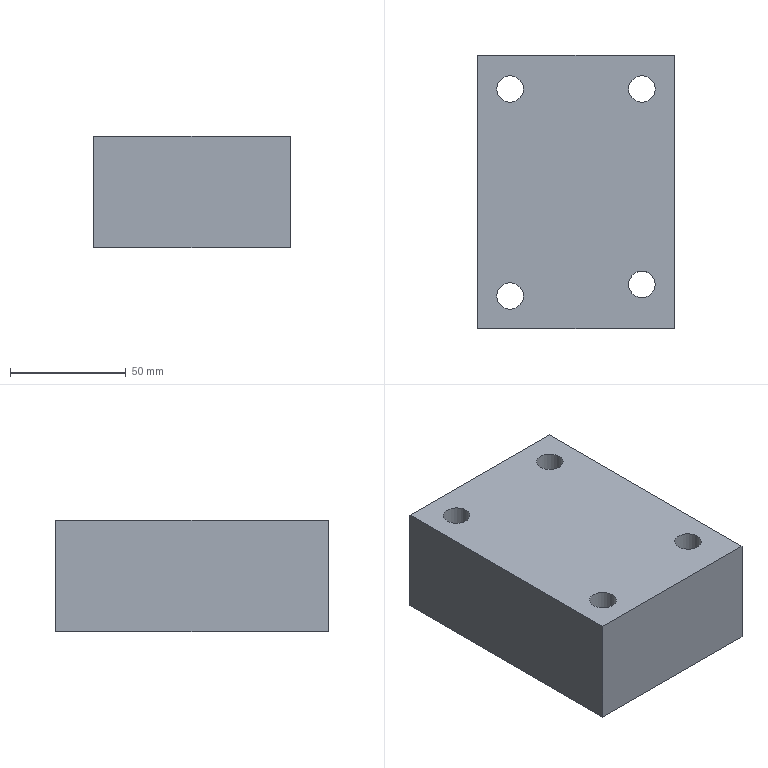Part | NX | features solid 2 | 1 solid | 35 faces | box 85 x 118 x 48 mm | volume 417820 mm3 | cylinder 16 | plane 15 | cone 4 | commonest cylinder face diameters 10 x4 11.509 x4 18.007 x4 8.5 x2 8.506 x2
STEP:
#1=CARTESIAN_POINT('',(1168.789,-205.654,50.));
#2=VERTEX_POINT('',#1);
#3=CARTESIAN_POINT('',(1159.786,-205.654,50.));
#4=DIRECTION('',(0.,0.,-1.));
#5=DIRECTION('',(1.,0.,0.));
#6=AXIS2_PLACEMENT_3D('',#3,#4,#5);
#7=CIRCLE('',#6,9.004);
#8=EDGE_CURVE('',#2,#2,#7,.T.);
#9=ORIENTED_EDGE('',*,*,#8,.F.);
#10=EDGE_LOOP('',(#9));
#11=FACE_BOUND('',#10,.T.);
#12=CARTESIAN_POINT('',(1225.789,-116.154,50.));
#13=VERTEX_POINT('',#12);
#14=CARTESIAN_POINT('',(1216.786,-116.154,50.));
#15=DIRECTION('',(0.,0.,-1.));
#16=DIRECTION('',(1.,0.,0.));
#17=AXIS2_PLACEMENT_3D('',#14,#15,#16);
#18=CIRCLE('',#17,9.004);
#19=EDGE_CURVE('',#13,#13,#18,.T.);
#20=ORIENTED_EDGE('',*,*,#19,.F.);
#21=EDGE_LOOP('',(#20));
#22=FACE_BOUND('',#21,.T.);
#23=CARTESIAN_POINT('',(1230.786,-219.654,50.));
#24=VERTEX_POINT('',#23);
#25=CARTESIAN_POINT('',(1145.786,-219.654,50.));
#26=VERTEX_POINT('',#25);
#27=CARTESIAN_POINT('',(1188.286,-219.654,50.));
#28=DIRECTION('',(-1.,0.,0.));
#29=VECTOR('',#28,1000.);
#30=LINE('',#27,#29);
#31=EDGE_CURVE('',#24,#26,#30,.T.);
#32=ORIENTED_EDGE('',*,*,#31,.T.);
#33=CARTESIAN_POINT('',(1145.786,-101.654,50.));
#34=VERTEX_POINT('',#33);
#35=CARTESIAN_POINT('',(1145.786,0.,50.));
#36=DIRECTION('',(0.,-1.,0.));
#37=VECTOR('',#36,1000.);
#38=LINE('',#35,#37);
#39=EDGE_CURVE('',#34,#26,#38,.T.);
#40=ORIENTED_EDGE('',*,*,#39,.F.);
#41=CARTESIAN_POINT('',(1230.786,-101.654,50.));
#42=VERTEX_POINT('',#41);
#43=CARTESIAN_POINT('',(1188.286,-101.654,50.));
#44=DIRECTION('',(-1.,0.,0.));
#45=VECTOR('',#44,1000.);
#46=LINE('',#43,#45);
#47=EDGE_CURVE('',#42,#34,#46,.T.);
#48=ORIENTED_EDGE('',*,*,#47,.F.);
#49=CARTESIAN_POINT('',(1230.786,0.,50.));
#50=DIRECTION('',(0.,1.,0.));
#51=VECTOR('',#50,1000.);
#52=LINE('',#49,#51);
#53=EDGE_CURVE('',#24,#42,#52,.T.);
#54=ORIENTED_EDGE('',*,*,#53,.F.);
#55=EDGE_LOOP('',(#32,#40,#48,#54));
#56=FACE_BOUND('',#55,.T.);
#57=CARTESIAN_POINT('',(1225.789,-200.654,50.));
#58=VERTEX_POINT('',#57);
#59=CARTESIAN_POINT('',(1216.786,-200.654,50.));
#60=DIRECTION('',(0.,0.,-1.));
#61=DIRECTION('',(1.,0.,0.));
#62=AXIS2_PLACEMENT_3D('',#59,#60,#61);
#63=CIRCLE('',#62,9.004);
#64=EDGE_CURVE('',#58,#58,#63,.T.);
#65=ORIENTED_EDGE('',*,*,#64,.F.);
#66=EDGE_LOOP('',(#65));
#67=FACE_BOUND('',#66,.T.);
#68=CARTESIAN_POINT('',(1168.789,-116.154,50.));
#69=VERTEX_POINT('',#68);
#70=CARTESIAN_POINT('',(1159.786,-116.154,50.));
#71=DIRECTION('',(0.,0.,-1.));
#72=DIRECTION('',(1.,0.,0.));
#73=AXIS2_PLACEMENT_3D('',#70,#71,#72);
#74=CIRCLE('',#73,9.004);
#75=EDGE_CURVE('',#69,#69,#74,.T.);
#76=ORIENTED_EDGE('',*,*,#75,.F.);
#77=EDGE_LOOP('',(#76));
#78=FACE_BOUND('',#77,.T.);
#79=CARTESIAN_POINT('',(1156.536,-159.154,50.));
#80=VERTEX_POINT('',#79);
#81=CARTESIAN_POINT('',(1160.786,-159.154,50.));
#82=DIRECTION('',(0.,0.,1.));
#83=DIRECTION('',(-1.,0.,0.));
#84=AXIS2_PLACEMENT_3D('',#81,#82,#83);
#85=CIRCLE('',#84,4.25);
#86=EDGE_CURVE('',#80,#80,#85,.T.);
#87=ORIENTED_EDGE('',*,*,#86,.T.);
#88=EDGE_LOOP('',(#87));
#89=FACE_BOUND('',#88,.T.);
#90=CARTESIAN_POINT('',(1211.536,-159.154,50.));
#91=VERTEX_POINT('',#90);
#92=CARTESIAN_POINT('',(1215.786,-159.154,50.));
#93=DIRECTION('',(0.,0.,1.));
#94=DIRECTION('',(-1.,0.,0.));
#95=AXIS2_PLACEMENT_3D('',#92,#93,#94);
#96=CIRCLE('',#95,4.25);
#97=EDGE_CURVE('',#91,#91,#96,.T.);
#98=ORIENTED_EDGE('',*,*,#97,.T.);
#99=EDGE_LOOP('',(#98));
#100=FACE_BOUND('',#99,.T.);
#101=CARTESIAN_POINT('',(1206.996,-131.014,50.));
#102=VERTEX_POINT('',#101);
#103=CARTESIAN_POINT('',(1199.996,-124.014,50.));
#104=VERTEX_POINT('',#103);
#105=CARTESIAN_POINT('',(1203.996,-127.014,50.));
#106=DIRECTION('',(0.,0.,1.));
#107=DIRECTION('',(-1.,0.,0.));
#108=AXIS2_PLACEMENT_3D('',#105,#106,#107);
#109=CIRCLE('',#108,5.);
#110=EDGE_CURVE('',#102,#104,#109,.T.);
#111=ORIENTED_EDGE('',*,*,#110,.T.);
#112=CARTESIAN_POINT('',(1176.576,-124.014,50.));
#113=VERTEX_POINT('',#112);
#114=CARTESIAN_POINT('',(1127.,-124.014,50.));
#115=DIRECTION('',(1.,0.,0.));
#116=VECTOR('',#115,1000.);
#117=LINE('',#114,#116);
#118=EDGE_CURVE('',#113,#104,#117,.T.);
#119=ORIENTED_EDGE('',*,*,#118,.F.);
#120=CARTESIAN_POINT('',(1169.576,-131.014,50.));
#121=VERTEX_POINT('',#120);
#122=CARTESIAN_POINT('',(1172.576,-127.014,50.));
#123=DIRECTION('',(0.,0.,1.));
#124=DIRECTION('',(-1.,0.,0.));
#125=AXIS2_PLACEMENT_3D('',#122,#123,#124);
#126=CIRCLE('',#125,5.);
#127=EDGE_CURVE('',#113,#121,#126,.T.);
#128=ORIENTED_EDGE('',*,*,#127,.T.);
#129=CARTESIAN_POINT('',(1169.576,-187.154,50.));
#130=VERTEX_POINT('',#129);
#131=CARTESIAN_POINT('',(1169.576,0.,50.));
#132=DIRECTION('',(0.,1.,0.));
#133=VECTOR('',#132,1000.);
#134=LINE('',#131,#133);
#135=EDGE_CURVE('',#130,#121,#134,.T.);
#136=ORIENTED_EDGE('',*,*,#135,.F.);
#137=CARTESIAN_POINT('',(1176.576,-194.154,50.));
#138=VERTEX_POINT('',#137);
#139=CARTESIAN_POINT('',(1172.576,-191.154,50.));
#140=DIRECTION('',(0.,0.,1.));
#141=DIRECTION('',(-1.,0.,0.));
#142=AXIS2_PLACEMENT_3D('',#139,#140,#141);
#143=CIRCLE('',#142,5.);
#144=EDGE_CURVE('',#130,#138,#143,.T.);
#145=ORIENTED_EDGE('',*,*,#144,.T.);
#146=CARTESIAN_POINT('',(1199.996,-194.154,50.));
#147=VERTEX_POINT('',#146);
#148=CARTESIAN_POINT('',(1127.,-194.154,50.));
#149=DIRECTION('',(-1.,0.,0.));
#150=VECTOR('',#149,1000.);
#151=LINE('',#148,#150);
#152=EDGE_CURVE('',#147,#138,#151,.T.);
#153=ORIENTED_EDGE('',*,*,#152,.F.);
#154=CARTESIAN_POINT('',(1206.996,-187.154,50.));
#155=VERTEX_POINT('',#154);
#156=CARTESIAN_POINT('',(1203.996,-191.154,50.));
#157=DIRECTION('',(0.,0.,1.));
#158=DIRECTION('',(-1.,0.,0.));
#159=AXIS2_PLACEMENT_3D('',#156,#157,#158);
#160=CIRCLE('',#159,5.);
#161=EDGE_CURVE('',#155,#147,#160,.F.);
#162=ORIENTED_EDGE('',*,*,#161,.F.);
#163=CARTESIAN_POINT('',(1206.996,0.,50.));
#164=DIRECTION('',(0.,-1.,0.));
#165=VECTOR('',#164,1000.);
#166=LINE('',#163,#165);
#167=EDGE_CURVE('',#102,#155,#166,.T.);
#168=ORIENTED_EDGE('',*,*,#167,.F.);
#169=EDGE_LOOP('',(#111,#119,#128,#136,#145,#153,#162,#168));
#170=FACE_BOUND('',#169,.T.);
#171=CARTESIAN_POINT('',(1127.,0.,50.));
#172=DIRECTION('',(0.,0.,-1.));
#173=DIRECTION('',(-1.,0.,0.));
#174=AXIS2_PLACEMENT_3D('',#171,#172,#173);
#175=PLANE('',#174);
#176=ADVANCED_FACE('',(#11,#22,#56,#67,#78,#89,#100,#170),#175,.T.);
#177=CARTESIAN_POINT('',(1230.786,-101.654,98.));
#178=VERTEX_POINT('',#177);
#179=CARTESIAN_POINT('',(1230.786,-219.654,98.));
#180=VERTEX_POINT('',#179);
#181=CARTESIAN_POINT('',(1230.786,0.,98.));
#182=DIRECTION('',(0.,-1.,0.));
#183=VECTOR('',#182,1000.);
#184=LINE('',#181,#183);
#185=EDGE_CURVE('',#178,#180,#184,.T.);
#186=ORIENTED_EDGE('',*,*,#185,.T.);
#187=CARTESIAN_POINT('',(1230.786,-219.654,-52.75));
#188=DIRECTION('',(0.,0.,-1.));
#189=VECTOR('',#188,1000.);
#190=LINE('',#187,#189);
#191=EDGE_CURVE('',#180,#24,#190,.T.);
#192=ORIENTED_EDGE('',*,*,#191,.T.);
#193=ORIENTED_EDGE('',*,*,#53,.T.);
#194=CARTESIAN_POINT('',(1230.786,-101.654,50.));
#195=DIRECTION('',(0.,0.,1.));
#196=VECTOR('',#195,1000.);
#197=LINE('',#194,#196);
#198=EDGE_CURVE('',#42,#178,#197,.T.);
#199=ORIENTED_EDGE('',*,*,#198,.T.);
#200=EDGE_LOOP('',(#186,#192,#193,#199));
#201=FACE_BOUND('',#200,.T.);
#202=CARTESIAN_POINT('',(1230.786,-216.654,50.));
#203=DIRECTION('',(1.,0.,0.));
#204=DIRECTION('',(0.,0.,-1.));
#205=AXIS2_PLACEMENT_3D('',#202,#203,#204);
#206=PLANE('',#205);
#207=ADVANCED_FACE('',(#201),#206,.T.);
#208=CARTESIAN_POINT('',(1165.54,-205.654,98.));
#209=VERTEX_POINT('',#208);
#210=CARTESIAN_POINT('',(1159.786,-205.654,98.));
#211=DIRECTION('',(0.,0.,-1.));
#212=DIRECTION('',(1.,0.,0.));
#213=AXIS2_PLACEMENT_3D('',#210,#211,#212);
#214=CIRCLE('',#213,5.755);
#215=EDGE_CURVE('',#209,#209,#214,.T.);
#216=ORIENTED_EDGE('',*,*,#215,.T.);
#217=EDGE_LOOP('',(#216));
#218=FACE_BOUND('',#217,.T.);
#219=CARTESIAN_POINT('',(1165.54,-116.154,98.));
#220=VERTEX_POINT('',#219);
#221=CARTESIAN_POINT('',(1159.786,-116.154,98.));
#222=DIRECTION('',(0.,0.,-1.));
#223=DIRECTION('',(1.,0.,0.));
#224=AXIS2_PLACEMENT_3D('',#221,#222,#223);
#225=CIRCLE('',#224,5.755);
#226=EDGE_CURVE('',#220,#220,#225,.T.);
#227=ORIENTED_EDGE('',*,*,#226,.T.);
#228=EDGE_LOOP('',(#227));
#229=FACE_BOUND('',#228,.T.);
#230=CARTESIAN_POINT('',(1222.54,-116.154,98.));
#231=VERTEX_POINT('',#230);
#232=CARTESIAN_POINT('',(1216.786,-116.154,98.));
#233=DIRECTION('',(0.,0.,-1.));
#234=DIRECTION('',(1.,0.,0.));
#235=AXIS2_PLACEMENT_3D('',#232,#233,#234);
#236=CIRCLE('',#235,5.755);
#237=EDGE_CURVE('',#231,#231,#236,.T.);
#238=ORIENTED_EDGE('',*,*,#237,.T.);
#239=EDGE_LOOP('',(#238));
#240=FACE_BOUND('',#239,.T.);
#241=CARTESIAN_POINT('',(1222.54,-200.654,98.));
#242=VERTEX_POINT('',#241);
#243=CARTESIAN_POINT('',(1216.786,-200.654,98.));
#244=DIRECTION('',(0.,0.,-1.));
#245=DIRECTION('',(1.,0.,0.));
#246=AXIS2_PLACEMENT_3D('',#243,#244,#245);
#247=CIRCLE('',#246,5.755);
#248=EDGE_CURVE('',#242,#242,#247,.T.);
#249=ORIENTED_EDGE('',*,*,#248,.T.);
#250=EDGE_LOOP('',(#249));
#251=FACE_BOUND('',#250,.T.);
#252=CARTESIAN_POINT('',(1145.786,-101.654,98.));
#253=VERTEX_POINT('',#252);
#254=CARTESIAN_POINT('',(835.5,-101.654,98.));
#255=DIRECTION('',(-1.,0.,0.));
#256=VECTOR('',#255,1000.);
#257=LINE('',#254,#256);
#258=EDGE_CURVE('',#178,#253,#257,.T.);
#259=ORIENTED_EDGE('',*,*,#258,.T.);
#260=CARTESIAN_POINT('',(1145.786,-219.654,98.));
#261=VERTEX_POINT('',#260);
#262=CARTESIAN_POINT('',(1145.786,0.,98.));
#263=DIRECTION('',(0.,1.,0.));
#264=VECTOR('',#263,1000.);
#265=LINE('',#262,#264);
#266=EDGE_CURVE('',#261,#253,#265,.T.);
#267=ORIENTED_EDGE('',*,*,#266,.F.);
#268=CARTESIAN_POINT('',(1188.286,-219.654,98.));
#269=DIRECTION('',(1.,0.,0.));
#270=VECTOR('',#269,1000.);
#271=LINE('',#268,#270);
#272=EDGE_CURVE('',#261,#180,#271,.T.);
#273=ORIENTED_EDGE('',*,*,#272,.T.);
#274=ORIENTED_EDGE('',*,*,#185,.F.);
#275=EDGE_LOOP('',(#259,#267,#273,#274));
#276=FACE_BOUND('',#275,.T.);
#277=CARTESIAN_POINT('',(835.5,0.,98.));
#278=DIRECTION('',(0.,0.,1.));
#279=DIRECTION('',(1.,0.,0.));
#280=AXIS2_PLACEMENT_3D('',#277,#278,#279);
#281=PLANE('',#280);
#282=ADVANCED_FACE('',(#218,#229,#240,#251,#276),#281,.T.);
#283=ORIENTED_EDGE('',*,*,#47,.T.);
#284=CARTESIAN_POINT('',(1145.786,-101.654,50.));
#285=DIRECTION('',(0.,0.,-1.));
#286=VECTOR('',#285,1000.);
#287=LINE('',#284,#286);
#288=EDGE_CURVE('',#253,#34,#287,.T.);
#289=ORIENTED_EDGE('',*,*,#288,.F.);
#290=ORIENTED_EDGE('',*,*,#258,.F.);
#291=ORIENTED_EDGE('',*,*,#198,.F.);
#292=EDGE_LOOP('',(#283,#289,#290,#291));
#293=FACE_BOUND('',#292,.T.);
#294=CARTESIAN_POINT('',(1188.286,-101.654,87.75));
#295=DIRECTION('',(0.,1.,0.));
#296=DIRECTION('',(0.,0.,-1.));
#297=AXIS2_PLACEMENT_3D('',#294,#295,#296);
#298=PLANE('',#297);
#299=ADVANCED_FACE('',(#293),#298,.T.);
#300=ORIENTED_EDGE('',*,*,#272,.F.);
#301=CARTESIAN_POINT('',(1145.786,-219.654,-52.75));
#302=DIRECTION('',(0.,0.,1.));
#303=VECTOR('',#302,1000.);
#304=LINE('',#301,#303);
#305=EDGE_CURVE('',#26,#261,#304,.T.);
#306=ORIENTED_EDGE('',*,*,#305,.F.);
#307=ORIENTED_EDGE('',*,*,#31,.F.);
#308=ORIENTED_EDGE('',*,*,#191,.F.);
#309=EDGE_LOOP('',(#300,#306,#307,#308));
#310=FACE_BOUND('',#309,.T.);
#311=CARTESIAN_POINT('',(1188.286,-219.654,-52.75));
#312=DIRECTION('',(0.,-1.,0.));
#313=DIRECTION('',(0.,0.,1.));
#314=AXIS2_PLACEMENT_3D('',#311,#312,#313);
#315=PLANE('',#314);
#316=ADVANCED_FACE('',(#310),#315,.T.);
#317=ORIENTED_EDGE('',*,*,#266,.T.);
#318=ORIENTED_EDGE('',*,*,#288,.T.);
#319=ORIENTED_EDGE('',*,*,#39,.T.);
#320=ORIENTED_EDGE('',*,*,#305,.T.);
#321=EDGE_LOOP('',(#317,#318,#319,#320));
#322=FACE_BOUND('',#321,.T.);
#323=CARTESIAN_POINT('',(1145.786,-216.654,50.));
#324=DIRECTION('',(-1.,0.,0.));
#325=DIRECTION('',(0.,0.,1.));
#326=AXIS2_PLACEMENT_3D('',#323,#324,#325);
#327=PLANE('',#326);
#328=ADVANCED_FACE('',(#322),#327,.T.);
#329=ORIENTED_EDGE('',*,*,#248,.F.);
#330=EDGE_LOOP('',(#329));
#331=FACE_BOUND('',#330,.T.);
#332=CARTESIAN_POINT('',(1222.54,-200.654,68.));
#333=VERTEX_POINT('',#332);
#334=CARTESIAN_POINT('',(1216.786,-200.654,68.));
#335=DIRECTION('',(0.,0.,-1.));
#336=DIRECTION('',(1.,0.,0.));
#337=AXIS2_PLACEMENT_3D('',#334,#335,#336);
#338=CIRCLE('',#337,5.755);
#339=EDGE_CURVE('',#333,#333,#338,.T.);
#340=ORIENTED_EDGE('',*,*,#339,.T.);
#341=EDGE_LOOP('',(#340));
#342=FACE_BOUND('',#341,.T.);
#343=CARTESIAN_POINT('',(1216.786,-200.654,45.));
#344=DIRECTION('',(0.,0.,1.));
#345=DIRECTION('',(1.,0.,0.));
#346=AXIS2_PLACEMENT_3D('',#343,#344,#345);
#347=CYLINDRICAL_SURFACE('',#346,5.755);
#348=ADVANCED_FACE('',(#331,#342),#347,.F.);
#349=ORIENTED_EDGE('',*,*,#339,.F.);
#350=EDGE_LOOP('',(#349));
#351=FACE_BOUND('',#350,.T.);
#352=CARTESIAN_POINT('',(1225.789,-200.654,68.));
#353=VERTEX_POINT('',#352);
#354=CARTESIAN_POINT('',(1216.786,-200.654,68.));
#355=DIRECTION('',(0.,0.,1.));
#356=DIRECTION('',(1.,0.,0.));
#357=AXIS2_PLACEMENT_3D('',#354,#355,#356);
#358=CIRCLE('',#357,9.004);
#359=EDGE_CURVE('',#353,#353,#358,.F.);
#360=ORIENTED_EDGE('',*,*,#359,.T.);
#361=EDGE_LOOP('',(#360));
#362=FACE_BOUND('',#361,.T.);
#363=CARTESIAN_POINT('',(1216.786,-200.654,68.));
#364=DIRECTION('',(0.,0.,1.));
#365=DIRECTION('',(1.,0.,0.));
#366=AXIS2_PLACEMENT_3D('',#363,#364,#365);
#367=PLANE('',#366);
#368=ADVANCED_FACE('',(#351,#362),#367,.F.);
#369=ORIENTED_EDGE('',*,*,#359,.F.);
#370=EDGE_LOOP('',(#369));
#371=FACE_BOUND('',#370,.T.);
#372=ORIENTED_EDGE('',*,*,#64,.T.);
#373=EDGE_LOOP('',(#372));
#374=FACE_BOUND('',#373,.T.);
#375=CARTESIAN_POINT('',(1216.786,-200.654,50.));
#376=DIRECTION('',(0.,0.,1.));
#377=DIRECTION('',(1.,0.,0.));
#378=AXIS2_PLACEMENT_3D('',#375,#376,#377);
#379=CYLINDRICAL_SURFACE('',#378,9.004);
#380=ADVANCED_FACE('',(#371,#374),#379,.F.);
#381=ORIENTED_EDGE('',*,*,#237,.F.);
#382=EDGE_LOOP('',(#381));
#383=FACE_BOUND('',#382,.T.);
#384=CARTESIAN_POINT('',(1222.54,-116.154,68.));
#385=VERTEX_POINT('',#384);
#386=CARTESIAN_POINT('',(1216.786,-116.154,68.));
#387=DIRECTION('',(0.,0.,-1.));
#388=DIRECTION('',(1.,0.,0.));
#389=AXIS2_PLACEMENT_3D('',#386,#387,#388);
#390=CIRCLE('',#389,5.755);
#391=EDGE_CURVE('',#385,#385,#390,.T.);
#392=ORIENTED_EDGE('',*,*,#391,.T.);
#393=EDGE_LOOP('',(#392));
#394=FACE_BOUND('',#393,.T.);
#395=CARTESIAN_POINT('',(1216.786,-116.154,45.));
#396=DIRECTION('',(0.,0.,1.));
#397=DIRECTION('',(1.,0.,0.));
#398=AXIS2_PLACEMENT_3D('',#395,#396,#397);
#399=CYLINDRICAL_SURFACE('',#398,5.755);
#400=ADVANCED_FACE('',(#383,#394),#399,.F.);
#401=ORIENTED_EDGE('',*,*,#391,.F.);
#402=EDGE_LOOP('',(#401));
#403=FACE_BOUND('',#402,.T.);
#404=CARTESIAN_POINT('',(1225.789,-116.154,68.));
#405=VERTEX_POINT('',#404);
#406=CARTESIAN_POINT('',(1216.786,-116.154,68.));
#407=DIRECTION('',(0.,0.,1.));
#408=DIRECTION('',(1.,0.,0.));
#409=AXIS2_PLACEMENT_3D('',#406,#407,#408);
#410=CIRCLE('',#409,9.004);
#411=EDGE_CURVE('',#405,#405,#410,.F.);
#412=ORIENTED_EDGE('',*,*,#411,.T.);
#413=EDGE_LOOP('',(#412));
#414=FACE_BOUND('',#413,.T.);
#415=CARTESIAN_POINT('',(1216.786,-116.154,68.));
#416=DIRECTION('',(0.,0.,1.));
#417=DIRECTION('',(1.,0.,0.));
#418=AXIS2_PLACEMENT_3D('',#415,#416,#417);
#419=PLANE('',#418);
#420=ADVANCED_FACE('',(#403,#414),#419,.F.);
#421=ORIENTED_EDGE('',*,*,#411,.F.);
#422=EDGE_LOOP('',(#421));
#423=FACE_BOUND('',#422,.T.);
#424=ORIENTED_EDGE('',*,*,#19,.T.);
#425=EDGE_LOOP('',(#424));
#426=FACE_BOUND('',#425,.T.);
#427=CARTESIAN_POINT('',(1216.786,-116.154,50.));
#428=DIRECTION('',(0.,0.,1.));
#429=DIRECTION('',(1.,0.,0.));
#430=AXIS2_PLACEMENT_3D('',#427,#428,#429);
#431=CYLINDRICAL_SURFACE('',#430,9.004);
#432=ADVANCED_FACE('',(#423,#426),#431,.F.);
#433=ORIENTED_EDGE('',*,*,#226,.F.);
#434=EDGE_LOOP('',(#433));
#435=FACE_BOUND('',#434,.T.);
#436=CARTESIAN_POINT('',(1165.54,-116.154,68.));
#437=VERTEX_POINT('',#436);
#438=CARTESIAN_POINT('',(1159.786,-116.154,68.));
#439=DIRECTION('',(0.,0.,-1.));
#440=DIRECTION('',(1.,0.,0.));
#441=AXIS2_PLACEMENT_3D('',#438,#439,#440);
#442=CIRCLE('',#441,5.755);
#443=EDGE_CURVE('',#437,#437,#442,.T.);
#444=ORIENTED_EDGE('',*,*,#443,.T.);
#445=EDGE_LOOP('',(#444));
#446=FACE_BOUND('',#445,.T.);
#447=CARTESIAN_POINT('',(1159.786,-116.154,45.));
#448=DIRECTION('',(0.,0.,1.));
#449=DIRECTION('',(1.,0.,0.));
#450=AXIS2_PLACEMENT_3D('',#447,#448,#449);
#451=CYLINDRICAL_SURFACE('',#450,5.755);
#452=ADVANCED_FACE('',(#435,#446),#451,.F.);
#453=ORIENTED_EDGE('',*,*,#443,.F.);
#454=EDGE_LOOP('',(#453));
#455=FACE_BOUND('',#454,.T.);
#456=CARTESIAN_POINT('',(1168.789,-116.154,68.));
#457=VERTEX_POINT('',#456);
#458=CARTESIAN_POINT('',(1159.786,-116.154,68.));
#459=DIRECTION('',(0.,0.,1.));
#460=DIRECTION('',(1.,0.,0.));
#461=AXIS2_PLACEMENT_3D('',#458,#459,#460);
#462=CIRCLE('',#461,9.004);
#463=EDGE_CURVE('',#457,#457,#462,.F.);
#464=ORIENTED_EDGE('',*,*,#463,.T.);
#465=EDGE_LOOP('',(#464));
#466=FACE_BOUND('',#465,.T.);
#467=CARTESIAN_POINT('',(1159.786,-116.154,68.));
#468=DIRECTION('',(0.,0.,1.));
#469=DIRECTION('',(1.,0.,0.));
#470=AXIS2_PLACEMENT_3D('',#467,#468,#469);
#471=PLANE('',#470);
#472=ADVANCED_FACE('',(#455,#466),#471,.F.);
#473=ORIENTED_EDGE('',*,*,#463,.F.);
#474=EDGE_LOOP('',(#473));
#475=FACE_BOUND('',#474,.T.);
#476=ORIENTED_EDGE('',*,*,#75,.T.);
#477=EDGE_LOOP('',(#476));
#478=FACE_BOUND('',#477,.T.);
#479=CARTESIAN_POINT('',(1159.786,-116.154,50.));
#480=DIRECTION('',(0.,0.,1.));
#481=DIRECTION('',(1.,0.,0.));
#482=AXIS2_PLACEMENT_3D('',#479,#480,#481);
#483=CYLINDRICAL_SURFACE('',#482,9.004);
#484=ADVANCED_FACE('',(#475,#478),#483,.F.);
#485=ORIENTED_EDGE('',*,*,#215,.F.);
#486=EDGE_LOOP('',(#485));
#487=FACE_BOUND('',#486,.T.);
#488=CARTESIAN_POINT('',(1165.54,-205.654,68.));
#489=VERTEX_POINT('',#488);
#490=CARTESIAN_POINT('',(1159.786,-205.654,68.));
#491=DIRECTION('',(0.,0.,-1.));
#492=DIRECTION('',(1.,0.,0.));
#493=AXIS2_PLACEMENT_3D('',#490,#491,#492);
#494=CIRCLE('',#493,5.755);
#495=EDGE_CURVE('',#489,#489,#494,.T.);
#496=ORIENTED_EDGE('',*,*,#495,.T.);
#497=EDGE_LOOP('',(#496));
#498=FACE_BOUND('',#497,.T.);
#499=CARTESIAN_POINT('',(1159.786,-205.654,45.));
#500=DIRECTION('',(0.,0.,1.));
#501=DIRECTION('',(1.,0.,0.));
#502=AXIS2_PLACEMENT_3D('',#499,#500,#501);
#503=CYLINDRICAL_SURFACE('',#502,5.755);
#504=ADVANCED_FACE('',(#487,#498),#503,.F.);
#505=ORIENTED_EDGE('',*,*,#495,.F.);
#506=EDGE_LOOP('',(#505));
#507=FACE_BOUND('',#506,.T.);
#508=CARTESIAN_POINT('',(1168.789,-205.654,68.));
#509=VERTEX_POINT('',#508);
#510=CARTESIAN_POINT('',(1159.786,-205.654,68.));
#511=DIRECTION('',(0.,0.,1.));
#512=DIRECTION('',(1.,0.,0.));
#513=AXIS2_PLACEMENT_3D('',#510,#511,#512);
#514=CIRCLE('',#513,9.004);
#515=EDGE_CURVE('',#509,#509,#514,.F.);
#516=ORIENTED_EDGE('',*,*,#515,.T.);
#517=EDGE_LOOP('',(#516));
#518=FACE_BOUND('',#517,.T.);
#519=CARTESIAN_POINT('',(1159.786,-205.654,68.));
#520=DIRECTION('',(0.,0.,1.));
#521=DIRECTION('',(1.,0.,0.));
#522=AXIS2_PLACEMENT_3D('',#519,#520,#521);
#523=PLANE('',#522);
#524=ADVANCED_FACE('',(#507,#518),#523,.F.);
#525=ORIENTED_EDGE('',*,*,#515,.F.);
#526=EDGE_LOOP('',(#525));
#527=FACE_BOUND('',#526,.T.);
#528=ORIENTED_EDGE('',*,*,#8,.T.);
#529=EDGE_LOOP('',(#528));
#530=FACE_BOUND('',#529,.T.);
#531=CARTESIAN_POINT('',(1159.786,-205.654,50.));
#532=DIRECTION('',(0.,0.,1.));
#533=DIRECTION('',(1.,0.,0.));
#534=AXIS2_PLACEMENT_3D('',#531,#532,#533);
#535=CYLINDRICAL_SURFACE('',#534,9.004);
#536=ADVANCED_FACE('',(#527,#530),#535,.F.);
#537=CARTESIAN_POINT('',(1156.536,-159.154,70.));
#538=VERTEX_POINT('',#537);
#539=CARTESIAN_POINT('',(1160.786,-159.154,70.));
#540=DIRECTION('',(0.,0.,1.));
#541=DIRECTION('',(-1.,0.,0.));
#542=AXIS2_PLACEMENT_3D('',#539,#540,#541);
#543=CIRCLE('',#542,4.25);
#544=EDGE_CURVE('',#538,#538,#543,.F.);
#545=ORIENTED_EDGE('',*,*,#544,.T.);
#546=EDGE_LOOP('',(#545));
#547=FACE_BOUND('',#546,.T.);
#548=CARTESIAN_POINT('',(1160.786,-159.154,72.554));
#549=VERTEX_POINT('',#548);
#550=VERTEX_LOOP('',#549);
#551=FACE_BOUND('',#550,.T.);
#552=CARTESIAN_POINT('',(1160.786,-159.154,70.));
#553=DIRECTION('',(0.,0.,-1.));
#554=DIRECTION('',(1.,0.,0.));
#555=AXIS2_PLACEMENT_3D('',#552,#553,#554);
#556=CONICAL_SURFACE('',#555,4.25,1.03);
#557=ADVANCED_FACE('',(#547,#551),#556,.F.);
#558=ORIENTED_EDGE('',*,*,#86,.F.);
#559=EDGE_LOOP('',(#558));
#560=FACE_BOUND('',#559,.T.);
#561=ORIENTED_EDGE('',*,*,#544,.F.);
#562=EDGE_LOOP('',(#561));
#563=FACE_BOUND('',#562,.T.);
#564=CARTESIAN_POINT('',(1160.786,-159.154,50.));
#565=DIRECTION('',(0.,0.,1.));
#566=DIRECTION('',(-1.,0.,0.));
#567=AXIS2_PLACEMENT_3D('',#564,#565,#566);
#568=CYLINDRICAL_SURFACE('',#567,4.25);
#569=ADVANCED_FACE('',(#560,#563),#568,.F.);
#570=CARTESIAN_POINT('',(1220.036,-159.154,70.));
#571=VERTEX_POINT('',#570);
#572=CARTESIAN_POINT('',(1215.786,-159.154,70.));
#573=DIRECTION('',(0.,0.,-1.));
#574=DIRECTION('',(1.,0.,0.));
#575=AXIS2_PLACEMENT_3D('',#572,#573,#574);
#576=CIRCLE('',#575,4.25);
#577=EDGE_CURVE('',#571,#571,#576,.F.);
#578=ORIENTED_EDGE('',*,*,#577,.F.);
#579=EDGE_LOOP('',(#578));
#580=FACE_BOUND('',#579,.T.);
#581=CARTESIAN_POINT('',(1215.786,-159.154,72.554));
#582=VERTEX_POINT('',#581);
#583=VERTEX_LOOP('',#582);
#584=FACE_BOUND('',#583,.T.);
#585=CARTESIAN_POINT('',(1215.786,-159.154,70.));
#586=DIRECTION('',(0.,0.,-1.));
#587=DIRECTION('',(-1.,0.,0.));
#588=AXIS2_PLACEMENT_3D('',#585,#586,#587);
#589=CONICAL_SURFACE('',#588,4.25,1.03);
#590=ADVANCED_FACE('',(#580,#584),#589,.F.);
#591=ORIENTED_EDGE('',*,*,#97,.F.);
#592=EDGE_LOOP('',(#591));
#593=FACE_BOUND('',#592,.T.);
#594=ORIENTED_EDGE('',*,*,#577,.T.);
#595=EDGE_LOOP('',(#594));
#596=FACE_BOUND('',#595,.T.);
#597=CARTESIAN_POINT('',(1215.786,-159.154,50.));
#598=DIRECTION('',(0.,0.,1.));
#599=DIRECTION('',(1.,0.,0.));
#600=AXIS2_PLACEMENT_3D('',#597,#598,#599);
#601=CYLINDRICAL_SURFACE('',#600,4.25);
#602=ADVANCED_FACE('',(#593,#596),#601,.F.);
#603=CARTESIAN_POINT('',(1206.996,-131.014,60.));
#604=VERTEX_POINT('',#603);
#605=CARTESIAN_POINT('',(1206.996,-131.014,-87.));
#606=DIRECTION('',(0.,0.,1.));
#607=VECTOR('',#606,1000.);
#608=LINE('',#605,#607);
#609=EDGE_CURVE('',#604,#102,#608,.F.);
#610=ORIENTED_EDGE('',*,*,#609,.T.);
#611=ORIENTED_EDGE('',*,*,#167,.T.);
#612=CARTESIAN_POINT('',(1206.996,-187.154,60.));
#613=VERTEX_POINT('',#612);
#614=CARTESIAN_POINT('',(1206.996,-187.154,-87.));
#615=DIRECTION('',(0.,0.,1.));
#616=VECTOR('',#615,1000.);
#617=LINE('',#614,#616);
#618=EDGE_CURVE('',#613,#155,#617,.F.);
#619=ORIENTED_EDGE('',*,*,#618,.F.);
#620=CARTESIAN_POINT('',(1206.996,0.,60.));
#621=DIRECTION('',(0.,-1.,0.));
#622=VECTOR('',#621,1000.);
#623=LINE('',#620,#622);
#624=EDGE_CURVE('',#613,#604,#623,.F.);
#625=ORIENTED_EDGE('',*,*,#624,.T.);
#626=EDGE_LOOP('',(#610,#611,#619,#625));
#627=FACE_BOUND('',#626,.T.);
#628=CARTESIAN_POINT('',(1206.996,0.,-87.));
#629=DIRECTION('',(-1.,0.,0.));
#630=DIRECTION('',(0.,0.,1.));
#631=AXIS2_PLACEMENT_3D('',#628,#629,#630);
#632=PLANE('',#631);
#633=ADVANCED_FACE('',(#627),#632,.T.);
#634=ORIENTED_EDGE('',*,*,#110,.F.);
#635=ORIENTED_EDGE('',*,*,#609,.F.);
#636=CARTESIAN_POINT('',(1199.996,-124.014,60.));
#637=VERTEX_POINT('',#636);
#638=CARTESIAN_POINT('',(1203.996,-127.014,60.));
#639=DIRECTION('',(0.,0.,-1.));
#640=DIRECTION('',(1.,0.,0.));
#641=AXIS2_PLACEMENT_3D('',#638,#639,#640);
#642=CIRCLE('',#641,5.);
#643=EDGE_CURVE('',#637,#604,#642,.T.);
#644=ORIENTED_EDGE('',*,*,#643,.F.);
#645=CARTESIAN_POINT('',(1199.996,-124.014,-87.));
#646=DIRECTION('',(0.,0.,1.));
#647=VECTOR('',#646,1000.);
#648=LINE('',#645,#647);
#649=EDGE_CURVE('',#637,#104,#648,.F.);
#650=ORIENTED_EDGE('',*,*,#649,.T.);
#651=EDGE_LOOP('',(#634,#635,#644,#650));
#652=FACE_BOUND('',#651,.T.);
#653=CARTESIAN_POINT('',(1203.996,-127.014,-87.));
#654=DIRECTION('',(0.,0.,1.));
#655=DIRECTION('',(1.,0.,0.));
#656=AXIS2_PLACEMENT_3D('',#653,#654,#655);
#657=CYLINDRICAL_SURFACE('',#656,5.);
#658=ADVANCED_FACE('',(#652),#657,.F.);
#659=CARTESIAN_POINT('',(1176.576,-124.014,60.));
#660=VERTEX_POINT('',#659);
#661=CARTESIAN_POINT('',(1176.576,-124.014,-87.));
#662=DIRECTION('',(0.,0.,1.));
#663=VECTOR('',#662,1000.);
#664=LINE('',#661,#663);
#665=EDGE_CURVE('',#660,#113,#664,.F.);
#666=ORIENTED_EDGE('',*,*,#665,.T.);
#667=ORIENTED_EDGE('',*,*,#118,.T.);
#668=ORIENTED_EDGE('',*,*,#649,.F.);
#669=CARTESIAN_POINT('',(268.879,-124.014,60.));
#670=DIRECTION('',(1.,0.,0.));
#671=VECTOR('',#670,1000.);
#672=LINE('',#669,#671);
#673=EDGE_CURVE('',#637,#660,#672,.F.);
#674=ORIENTED_EDGE('',*,*,#673,.T.);
#675=EDGE_LOOP('',(#666,#667,#668,#674));
#676=FACE_BOUND('',#675,.T.);
#677=CARTESIAN_POINT('',(268.879,-124.014,-87.));
#678=DIRECTION('',(0.,-1.,0.));
#679=DIRECTION('',(0.,0.,1.));
#680=AXIS2_PLACEMENT_3D('',#677,#678,#679);
#681=PLANE('',#680);
#682=ADVANCED_FACE('',(#676),#681,.T.);
#683=ORIENTED_EDGE('',*,*,#127,.F.);
#684=ORIENTED_EDGE('',*,*,#665,.F.);
#685=CARTESIAN_POINT('',(1169.576,-131.014,60.));
#686=VERTEX_POINT('',#685);
#687=CARTESIAN_POINT('',(1172.576,-127.014,60.));
#688=DIRECTION('',(0.,0.,-1.));
#689=DIRECTION('',(1.,0.,0.));
#690=AXIS2_PLACEMENT_3D('',#687,#688,#689);
#691=CIRCLE('',#690,5.);
#692=EDGE_CURVE('',#686,#660,#691,.T.);
#693=ORIENTED_EDGE('',*,*,#692,.F.);
#694=CARTESIAN_POINT('',(1169.576,-131.014,-87.));
#695=DIRECTION('',(0.,0.,1.));
#696=VECTOR('',#695,1000.);
#697=LINE('',#694,#696);
#698=EDGE_CURVE('',#686,#121,#697,.F.);
#699=ORIENTED_EDGE('',*,*,#698,.T.);
#700=EDGE_LOOP('',(#683,#684,#693,#699));
#701=FACE_BOUND('',#700,.T.);
#702=CARTESIAN_POINT('',(1172.576,-127.014,-87.));
#703=DIRECTION('',(0.,0.,1.));
#704=DIRECTION('',(1.,0.,0.));
#705=AXIS2_PLACEMENT_3D('',#702,#703,#704);
#706=CYLINDRICAL_SURFACE('',#705,5.);
#707=ADVANCED_FACE('',(#701),#706,.F.);
#708=CARTESIAN_POINT('',(1169.576,-187.154,60.));
#709=VERTEX_POINT('',#708);
#710=CARTESIAN_POINT('',(1169.576,-187.154,-87.));
#711=DIRECTION('',(0.,0.,1.));
#712=VECTOR('',#711,1000.);
#713=LINE('',#710,#712);
#714=EDGE_CURVE('',#709,#130,#713,.F.);
#715=ORIENTED_EDGE('',*,*,#714,.T.);
#716=ORIENTED_EDGE('',*,*,#135,.T.);
#717=ORIENTED_EDGE('',*,*,#698,.F.);
#718=CARTESIAN_POINT('',(1169.576,0.,60.));
#719=DIRECTION('',(0.,1.,0.));
#720=VECTOR('',#719,1000.);
#721=LINE('',#718,#720);
#722=EDGE_CURVE('',#686,#709,#721,.F.);
#723=ORIENTED_EDGE('',*,*,#722,.T.);
#724=EDGE_LOOP('',(#715,#716,#717,#723));
#725=FACE_BOUND('',#724,.T.);
#726=CARTESIAN_POINT('',(1169.576,0.,-87.));
#727=DIRECTION('',(1.,0.,0.));
#728=DIRECTION('',(0.,0.,-1.));
#729=AXIS2_PLACEMENT_3D('',#726,#727,#728);
#730=PLANE('',#729);
#731=ADVANCED_FACE('',(#725),#730,.T.);
#732=ORIENTED_EDGE('',*,*,#144,.F.);
#733=ORIENTED_EDGE('',*,*,#714,.F.);
#734=CARTESIAN_POINT('',(1176.576,-194.154,60.));
#735=VERTEX_POINT('',#734);
#736=CARTESIAN_POINT('',(1172.576,-191.154,60.));
#737=DIRECTION('',(0.,0.,-1.));
#738=DIRECTION('',(1.,0.,0.));
#739=AXIS2_PLACEMENT_3D('',#736,#737,#738);
#740=CIRCLE('',#739,5.);
#741=EDGE_CURVE('',#735,#709,#740,.T.);
#742=ORIENTED_EDGE('',*,*,#741,.F.);
#743=CARTESIAN_POINT('',(1176.576,-194.154,-87.));
#744=DIRECTION('',(0.,0.,1.));
#745=VECTOR('',#744,1000.);
#746=LINE('',#743,#745);
#747=EDGE_CURVE('',#735,#138,#746,.F.);
#748=ORIENTED_EDGE('',*,*,#747,.T.);
#749=EDGE_LOOP('',(#732,#733,#742,#748));
#750=FACE_BOUND('',#749,.T.);
#751=CARTESIAN_POINT('',(1172.576,-191.154,-87.));
#752=DIRECTION('',(0.,0.,1.));
#753=DIRECTION('',(1.,0.,0.));
#754=AXIS2_PLACEMENT_3D('',#751,#752,#753);
#755=CYLINDRICAL_SURFACE('',#754,5.);
#756=ADVANCED_FACE('',(#750),#755,.F.);
#757=CARTESIAN_POINT('',(1199.996,-194.154,60.));
#758=VERTEX_POINT('',#757);
#759=CARTESIAN_POINT('',(1199.996,-194.154,-87.));
#760=DIRECTION('',(0.,0.,1.));
#761=VECTOR('',#760,1000.);
#762=LINE('',#759,#761);
#763=EDGE_CURVE('',#758,#147,#762,.F.);
#764=ORIENTED_EDGE('',*,*,#763,.T.);
#765=ORIENTED_EDGE('',*,*,#152,.T.);
#766=ORIENTED_EDGE('',*,*,#747,.F.);
#767=CARTESIAN_POINT('',(268.879,-194.154,60.));
#768=DIRECTION('',(-1.,0.,0.));
#769=VECTOR('',#768,1000.);
#770=LINE('',#767,#769);
#771=EDGE_CURVE('',#735,#758,#770,.F.);
#772=ORIENTED_EDGE('',*,*,#771,.T.);
#773=EDGE_LOOP('',(#764,#765,#766,#772));
#774=FACE_BOUND('',#773,.T.);
#775=CARTESIAN_POINT('',(268.879,-194.154,-87.));
#776=DIRECTION('',(0.,1.,0.));
#777=DIRECTION('',(0.,0.,-1.));
#778=AXIS2_PLACEMENT_3D('',#775,#776,#777);
#779=PLANE('',#778);
#780=ADVANCED_FACE('',(#774),#779,.T.);
#781=ORIENTED_EDGE('',*,*,#618,.T.);
#782=ORIENTED_EDGE('',*,*,#161,.T.);
#783=ORIENTED_EDGE('',*,*,#763,.F.);
#784=CARTESIAN_POINT('',(1203.996,-191.154,60.));
#785=DIRECTION('',(0.,0.,-1.));
#786=DIRECTION('',(1.,0.,0.));
#787=AXIS2_PLACEMENT_3D('',#784,#785,#786);
#788=CIRCLE('',#787,5.);
#789=EDGE_CURVE('',#758,#613,#788,.F.);
#790=ORIENTED_EDGE('',*,*,#789,.T.);
#791=EDGE_LOOP('',(#781,#782,#783,#790));
#792=FACE_BOUND('',#791,.T.);
#793=CARTESIAN_POINT('',(1203.996,-191.154,-87.));
#794=DIRECTION('',(0.,0.,1.));
#795=DIRECTION('',(1.,0.,0.));
#796=AXIS2_PLACEMENT_3D('',#793,#794,#795);
#797=CYLINDRICAL_SURFACE('',#796,5.);
#798=ADVANCED_FACE('',(#792),#797,.F.);
#799=CARTESIAN_POINT('',(1199.249,-183.154,60.));
#800=VERTEX_POINT('',#799);
#801=CARTESIAN_POINT('',(1194.996,-183.154,60.));
#802=DIRECTION('',(0.,0.,1.));
#803=DIRECTION('',(1.,0.,0.));
#804=AXIS2_PLACEMENT_3D('',#801,#802,#803);
#805=CIRCLE('',#804,4.253);
#806=EDGE_CURVE('',#800,#800,#805,.T.);
#807=ORIENTED_EDGE('',*,*,#806,.T.);
#808=EDGE_LOOP('',(#807));
#809=FACE_BOUND('',#808,.T.);
#810=CARTESIAN_POINT('',(1184.829,-169.154,60.));
#811=VERTEX_POINT('',#810);
#812=CARTESIAN_POINT('',(1180.576,-169.154,60.));
#813=DIRECTION('',(0.,0.,1.));
#814=DIRECTION('',(1.,0.,0.));
#815=AXIS2_PLACEMENT_3D('',#812,#813,#814);
#816=CIRCLE('',#815,4.253);
#817=EDGE_CURVE('',#811,#811,#816,.T.);
#818=ORIENTED_EDGE('',*,*,#817,.T.);
#819=EDGE_LOOP('',(#818));
#820=FACE_BOUND('',#819,.T.);
#821=ORIENTED_EDGE('',*,*,#643,.T.);
#822=ORIENTED_EDGE('',*,*,#624,.F.);
#823=ORIENTED_EDGE('',*,*,#789,.F.);
#824=ORIENTED_EDGE('',*,*,#771,.F.);
#825=ORIENTED_EDGE('',*,*,#741,.T.);
#826=ORIENTED_EDGE('',*,*,#722,.F.);
#827=ORIENTED_EDGE('',*,*,#692,.T.);
#828=ORIENTED_EDGE('',*,*,#673,.F.);
#829=EDGE_LOOP('',(#821,#822,#823,#824,#825,#826,#827,#828));
#830=FACE_BOUND('',#829,.T.);
#831=CARTESIAN_POINT('',(1188.286,-159.154,60.));
#832=DIRECTION('',(0.,0.,1.));
#833=DIRECTION('',(1.,0.,0.));
#834=AXIS2_PLACEMENT_3D('',#831,#832,#833);
#835=PLANE('',#834);
#836=ADVANCED_FACE('',(#809,#820,#830),#835,.F.);
#837=CARTESIAN_POINT('',(1176.323,-169.154,87.753));
#838=VERTEX_POINT('',#837);
#839=CARTESIAN_POINT('',(1180.576,-169.154,87.753));
#840=DIRECTION('',(0.,0.,-1.));
#841=DIRECTION('',(-1.,0.,0.));
#842=AXIS2_PLACEMENT_3D('',#839,#840,#841);
#843=CIRCLE('',#842,4.253);
#844=EDGE_CURVE('',#838,#838,#843,.T.);
#845=ORIENTED_EDGE('',*,*,#844,.F.);
#846=EDGE_LOOP('',(#845));
#847=FACE_BOUND('',#846,.T.);
#848=ORIENTED_EDGE('',*,*,#817,.F.);
#849=EDGE_LOOP('',(#848));
#850=FACE_BOUND('',#849,.T.);
#851=CARTESIAN_POINT('',(1180.576,-169.154,57.));
#852=DIRECTION('',(0.,0.,1.));
#853=DIRECTION('',(1.,0.,0.));
#854=AXIS2_PLACEMENT_3D('',#851,#852,#853);
#855=CYLINDRICAL_SURFACE('',#854,4.253);
#856=ADVANCED_FACE('',(#847,#850),#855,.F.);
#857=CARTESIAN_POINT('',(1180.576,-169.154,92.006));
#858=VERTEX_POINT('',#857);
#859=VERTEX_LOOP('',#858);
#860=FACE_BOUND('',#859,.T.);
#861=ORIENTED_EDGE('',*,*,#844,.T.);
#862=EDGE_LOOP('',(#861));
#863=FACE_BOUND('',#862,.T.);
#864=CARTESIAN_POINT('',(1180.576,-169.154,87.753));
#865=DIRECTION('',(0.,0.,-1.));
#866=DIRECTION('',(1.,0.,0.));
#867=AXIS2_PLACEMENT_3D('',#864,#865,#866);
#868=CONICAL_SURFACE('',#867,4.253,0.7854);
#869=ADVANCED_FACE('',(#860,#863),#868,.F.);
#870=CARTESIAN_POINT('',(1190.743,-183.154,87.753));
#871=VERTEX_POINT('',#870);
#872=CARTESIAN_POINT('',(1194.996,-183.154,87.753));
#873=DIRECTION('',(0.,0.,-1.));
#874=DIRECTION('',(-1.,0.,0.));
#875=AXIS2_PLACEMENT_3D('',#872,#873,#874);
#876=CIRCLE('',#875,4.253);
#877=EDGE_CURVE('',#871,#871,#876,.T.);
#878=ORIENTED_EDGE('',*,*,#877,.F.);
#879=EDGE_LOOP('',(#878));
#880=FACE_BOUND('',#879,.T.);
#881=ORIENTED_EDGE('',*,*,#806,.F.);
#882=EDGE_LOOP('',(#881));
#883=FACE_BOUND('',#882,.T.);
#884=CARTESIAN_POINT('',(1194.996,-183.154,57.));
#885=DIRECTION('',(0.,0.,1.));
#886=DIRECTION('',(1.,0.,0.));
#887=AXIS2_PLACEMENT_3D('',#884,#885,#886);
#888=CYLINDRICAL_SURFACE('',#887,4.253);
#889=ADVANCED_FACE('',(#880,#883),#888,.F.);
#890=CARTESIAN_POINT('',(1194.996,-183.154,92.006));
#891=VERTEX_POINT('',#890);
#892=VERTEX_LOOP('',#891);
#893=FACE_BOUND('',#892,.T.);
#894=ORIENTED_EDGE('',*,*,#877,.T.);
#895=EDGE_LOOP('',(#894));
#896=FACE_BOUND('',#895,.T.);
#897=CARTESIAN_POINT('',(1194.996,-183.154,87.753));
#898=DIRECTION('',(0.,0.,-1.));
#899=DIRECTION('',(1.,0.,0.));
#900=AXIS2_PLACEMENT_3D('',#897,#898,#899);
#901=CONICAL_SURFACE('',#900,4.253,0.7854);
#902=ADVANCED_FACE('',(#893,#896),#901,.F.);
#903=CLOSED_SHELL('',(#176,#207,#282,#299,#316,#328,#348,#368,#380,#400,#420,#432,#452,#472,#484,#504,#524,#536,#557,#569,#590,#602,#633,#658,#682,#707,#731,#756,#780,#798,#836,#856,#869,#889,#902));
#904=MANIFOLD_SOLID_BREP('',#903);
#905=(LENGTH_UNIT()NAMED_UNIT(*)SI_UNIT(.MILLI.,.METRE.));
#906=UNCERTAINTY_MEASURE_WITH_UNIT(LENGTH_MEASURE(0.00001),#905,'','');
#907=(NAMED_UNIT(*)PLANE_ANGLE_UNIT()SI_UNIT($,.RADIAN.));
#908=(NAMED_UNIT(*)SI_UNIT($,.STERADIAN.)SOLID_ANGLE_UNIT());
#909=(GEOMETRIC_REPRESENTATION_CONTEXT(3)GLOBAL_UNCERTAINTY_ASSIGNED_CONTEXT((#906))GLOBAL_UNIT_ASSIGNED_CONTEXT((#905,#907,#908))REPRESENTATION_CONTEXT('',''));
#910=ADVANCED_BREP_SHAPE_REPRESENTATION('',(#904),#909);